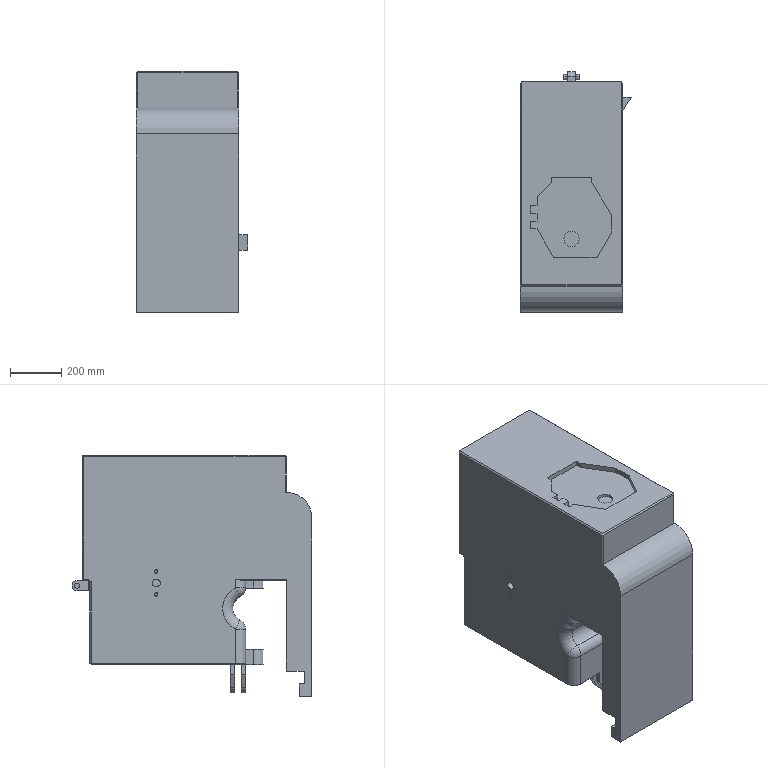Part | SolidWorks | 1 solid | 1312 faces | box 435.01 x 940 x 945 mm | volume 125087598 mm3 | cylinder 1115 | plane 155 | spline 34 | sphere 4 | torus 2 | cone 2 | commonest cylinder face diameters 10 x800 20 x254 12 x28 40 x9 80 x8 30 x4